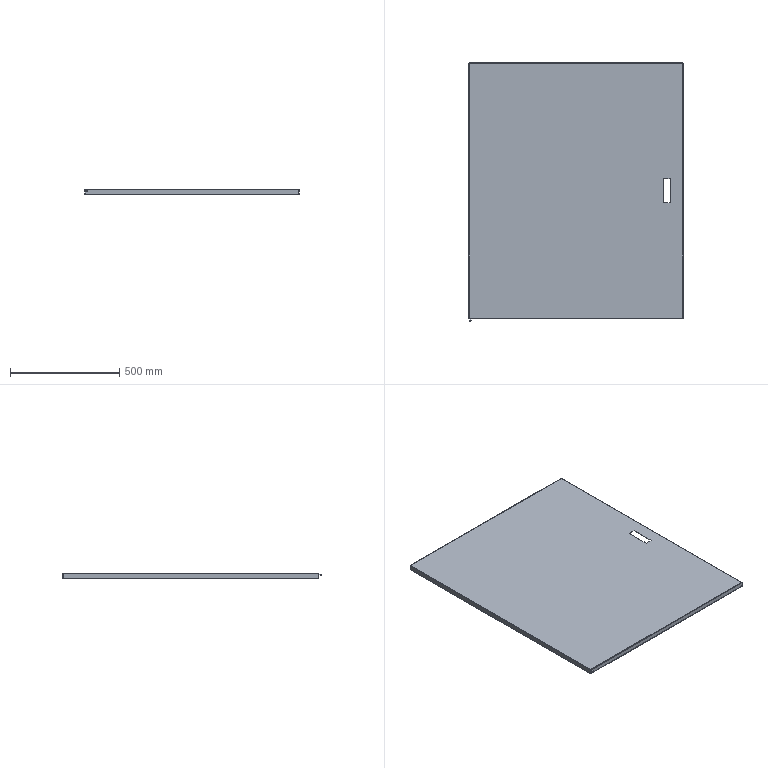Part | SolidWorks | features Cut 2, EdgeFlange 2, ICE 2, Chamfer 1, FlatPattern 1, SMBaseFlange 1, SheetMetal 1 | 1 solid | 85 faces | box 982 x 1182 x 24 mm | volume 1971875 mm3 | plane 45 | cylinder 22 | spline 16 | cone 2 | commonest cylinder face diameters 2 x8 5 x8 6 x2 7 x2 10 x2